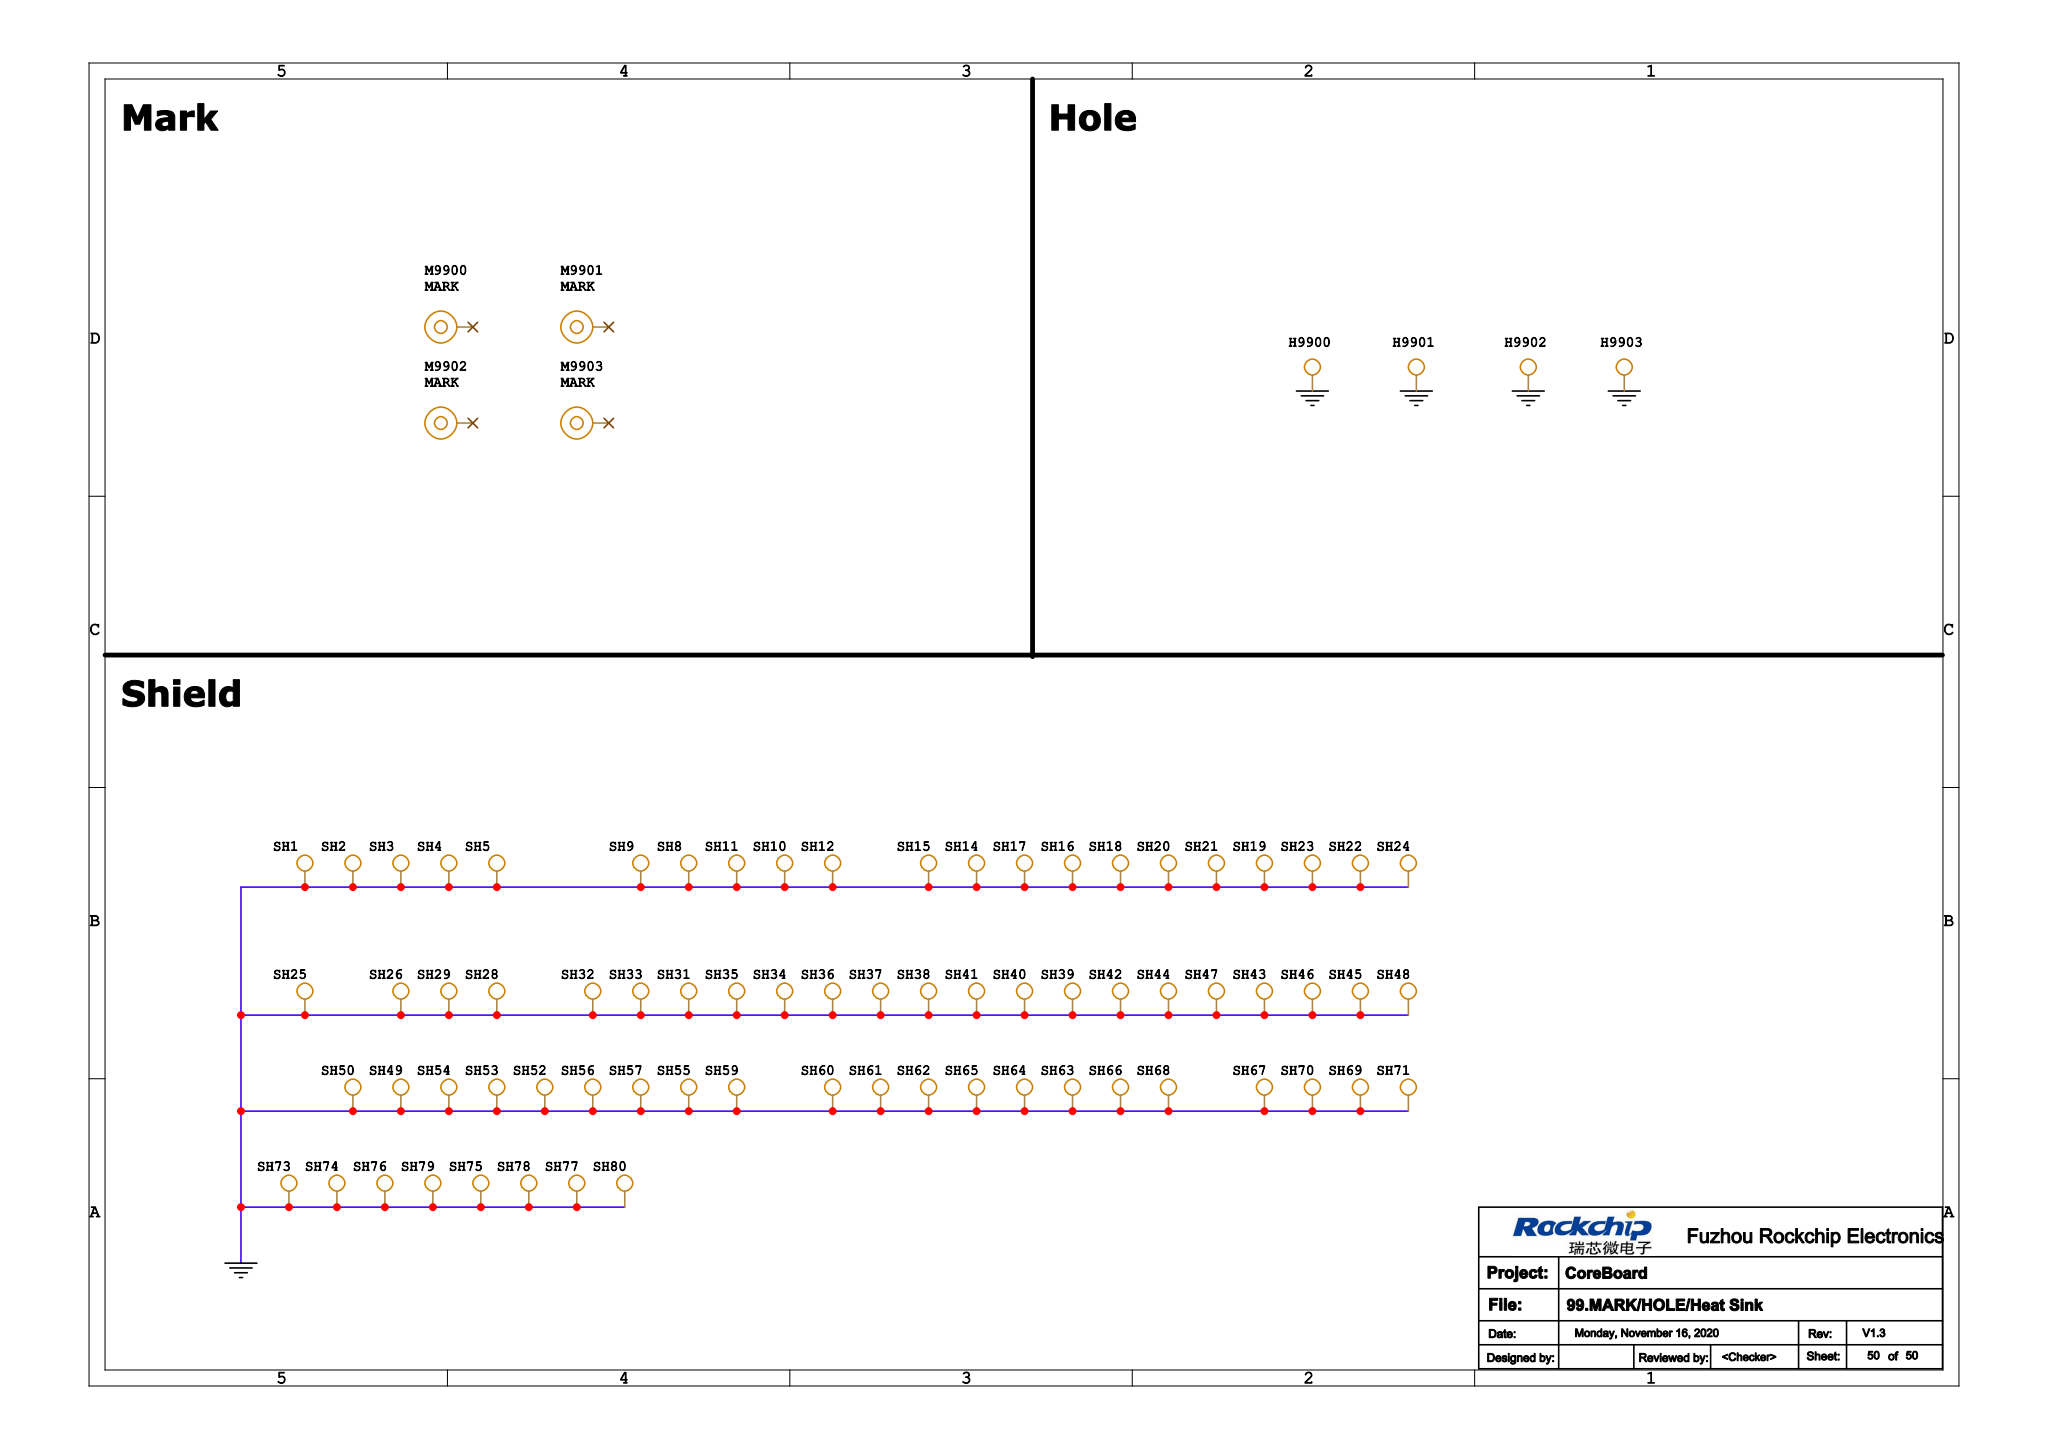Circuit board | Cadence Allegro | 749 parts | 717 nets | one sheet of the schematic
Parts on this sheet (reference | value | footprint):
H9900 | SHIELD | HOLE_4P5TH2P6
H9901 | SHIELD | HOLE_4P5TH2P6
H9902 | SHIELD | HOLE_4P5TH2P6
H9903 | SHIELD | HOLE_4P5TH2P6
SH1 | SHIELD | SHIELD_2X0P7
SH2 | SHIELD | SHIELD_2X0P7
SH3 | SHIELD | SHIELD_2X0P7
SH4 | SHIELD | SHIELD_2X0P7
SH5 | SHIELD | SHIELD_2X0P7
SH8 | SHIELD | SHIELD_2X0P7
SH9 | SHIELD | SHIELD_2X0P7
SH10 | SHIELD | SHIELD_2X0P7
SH11 | SHIELD | SHIELD_2X0P7
SH12 | SHIELD | SHIELD_2X0P7
SH14 | SHIELD | SHIELD_2X0P7
SH15 | SHIELD | SHIELD_2X0P7
SH16 | SHIELD | SHIELD_2X0P7
SH17 | SHIELD | SHIELD_2X0P7
SH18 | SHIELD | SHIELD_2X0P7
SH19 | SHIELD | SHIELD_2X0P7
SH20 | SHIELD | SHIELD_2X0P7
SH21 | SHIELD | SHIELD_2X0P7
SH22 | SHIELD | SHIELD_2X0P7
SH23 | SHIELD | SHIELD_2X0P7
SH24 | SHIELD | SHIELD_2X0P7
SH25 | SHIELD | SHIELD_2X0P7
SH26 | SHIELD | SHIELD_2X0P7
SH28 | SHIELD | SHIELD_2X0P7
SH29 | SHIELD | SHIELD_2X0P7
SH31 | SHIELD | SHIELD_2X0P7
SH32 | SHIELD | SHIELD_2X0P7
SH33 | SHIELD | SHIELD_2X0P7
SH34 | SHIELD | SHIELD_2X0P7
SH35 | SHIELD | SHIELD_2X0P7
SH36 | SHIELD | SHIELD_2X0P7
SH37 | SHIELD | SHIELD_2X0P7
SH38 | SHIELD | SHIELD_2X0P7
SH39 | SHIELD | SHIELD_2X0P7
SH40 | SHIELD | SHIELD_2X0P7
SH41 | SHIELD | SHIELD_2X0P7
SH42 | SHIELD | SHIELD_2X0P7
SH43 | SHIELD | SHIELD_2X0P7
SH44 | SHIELD | SHIELD_2X0P7
SH45 | SHIELD | SHIELD_2X0P7
SH46 | SHIELD | SHIELD_2X0P7
SH47 | SHIELD | SHIELD_2X0P7
SH48 | SHIELD | SHIELD_2X0P7
SH49 | SHIELD | SHIELD_2X0P7
SH50 | SHIELD | SHIELD_2X0P7
SH52 | SHIELD | SHIELD_2X0P7
SH53 | SHIELD | SHIELD_2X0P7
SH54 | SHIELD | SHIELD_2X0P7
SH55 | SHIELD | SHIELD_2X0P7
SH56 | SHIELD | SHIELD_2X0P7
SH57 | SHIELD | SHIELD_2X0P7
SH59 | SHIELD | SHIELD_2X0P7
SH60 | SHIELD | SHIELD_2X0P7
SH61 | SHIELD | SHIELD_2X0P7
SH62 | SHIELD | SHIELD_2X0P7
SH63 | SHIELD | SHIELD_2X0P7
SH64 | SHIELD | SHIELD_2X0P7
SH65 | SHIELD | SHIELD_2X0P7
SH66 | SHIELD | SHIELD_2X0P7
SH67 | SHIELD | SHIELD_2X0P7
SH68 | SHIELD | SHIELD_2X0P7
SH69 | SHIELD | SHIELD_2X0P7
SH70 | SHIELD | SHIELD_2X0P7
SH71 | SHIELD | SHIELD_2X0P7
SH73 | SHIELD | SHIELD_2X0P7
SH74 | SHIELD | SHIELD_2X0P7
SH75 | SHIELD | SHIELD_2X0P7
SH76 | SHIELD | SHIELD_2X0P7
SH77 | SHIELD | SHIELD_2X0P7
SH78 | SHIELD | SHIELD_2X0P7
SH79 | SHIELD | SHIELD_2X0P7
SH80 | SHIELD | SHIELD_2X0P7
Nets of these parts (net: part-pin ...):
GND: H9900-1 H9901-1 H9902-1 H9903-1 SH1-1 SH2-1 SH3-1 SH4-1 SH5-1 SH8-1 SH9-1 SH10-1 SH11-1 SH12-1 SH14-1 SH15-1 SH16-1 SH17-1 SH18-1 SH19-1 SH20-1 SH21-1 SH22-1 SH23-1 SH24-1 SH25-1 SH26-1 SH28-1 SH29-1 SH31-1 SH32-1 SH33-1 SH34-1 SH35-1 SH36-1 SH37-1 SH38-1 SH39-1 SH40-1 SH41-1 SH42-1 SH43-1 SH44-1 SH45-1 SH46-1 SH47-1 SH48-1 SH49-1 SH50-1 SH52-1 SH53-1 SH54-1 SH55-1 SH56-1 SH57-1 SH59-1 SH60-1 SH61-1 SH62-1 SH63-1 SH64-1 SH65-1 SH66-1 SH67-1 SH68-1 SH69-1 SH70-1 SH71-1 SH73-1 SH74-1 SH75-1 SH76-1 SH77-1 SH78-1 SH79-1 SH80-1